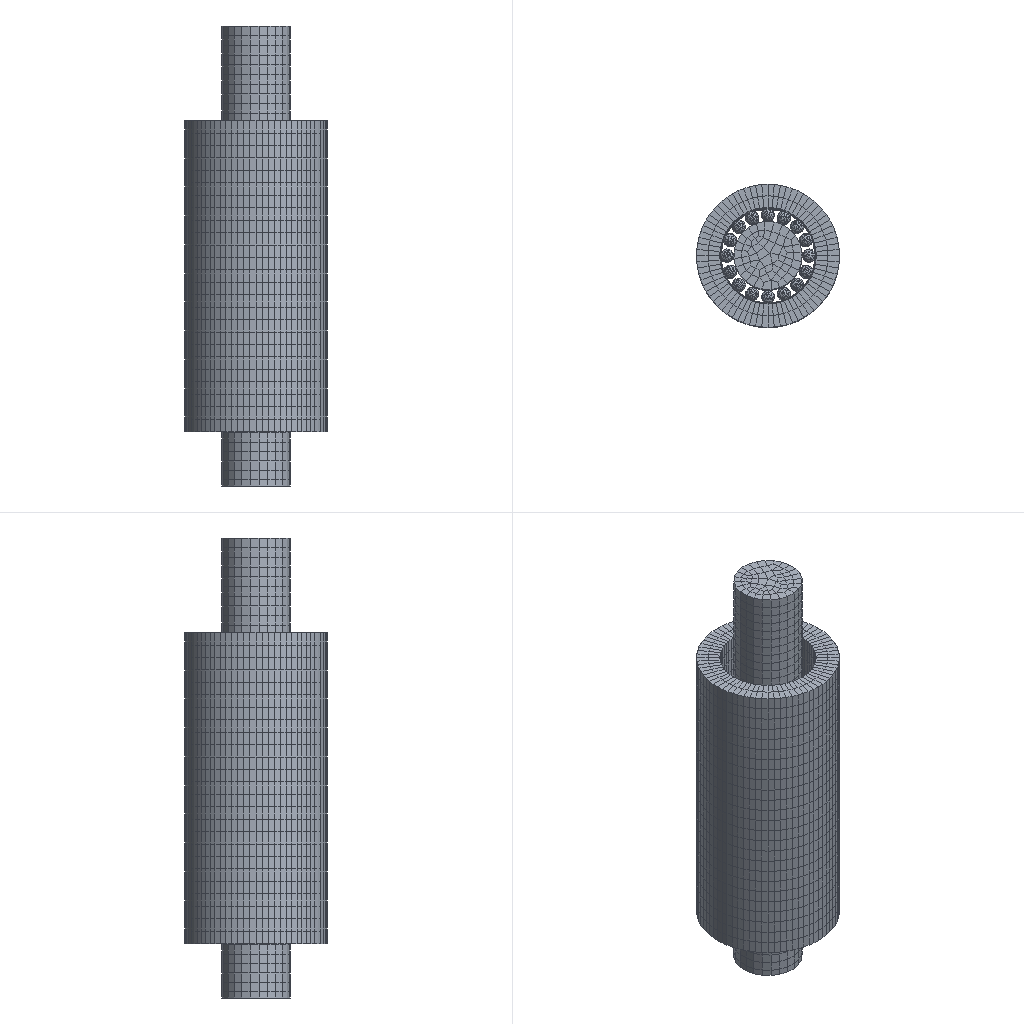Simulation study | abaqus
Set-up summary:
category,name,step,type,value,unit,region
solver,abaqus
solver,version,,,Abaqus/Explicit 2020
units,not stated in the deck,,not stated
analysis,deck,,transient,transient
load_step,Step-1,Step-1,transient
load_step,requested,,,1
mesh,nodes,,,38616
mesh,elements,,,24212
element_type,C3D10,,solid,17427
element_type,C3D8R,,solid,6785
load,load commands in deck,,count,1
bc,support commands in deck,,count,7
material,STEEL,,in results
material,TUBE,,in results
check,setup vs results,,match,"per instance, exact: element labels, types and connectivity; labels of the nodes the elements use; coordinates of those nodes at SINGLE_PRECISION in 2 of 34 instance(s)"
Abaqus input file, long lists of numbers shortened:
*Heading
** Job name: Job-1 Model name: Model-1
** Generated by: Abaqus/CAE 2020
*Preprint, echo=NO, model=NO, history=NO, contact=NO
**
** PARTS
**
*Part, name=work-1
*End Part
**
*Part, name=work-2
*End Part
**
*Part, name=work-3
*End Part
**
*Part, name=work-4
*End Part
**
*Part, name=work-5
*End Part
**
*Part, name=work-6
*End Part
**
*Part, name=work-7
*End Part
**
*Part, name=work-8
*End Part
**
*Part, name=work-9
*End Part
**
*Part, name=work-10
*End Part
**
*Part, name=work-11
*End Part
**
*Part, name=work-12
*End Part
**
*Part, name=work-13
*End Part
**
*Part, name=work-14
*End Part
**
*Part, name=work-15
*End Part
**
*Part, name=work-16
*End Part
**
*Part, name=work-19
*End Part
**
*Part, name=work-20
*End Part
**
*Part, name=work-21
*End Part
**
*Part, name=work-22
*End Part
**
*Part, name=work-23
*End Part
**
*Part, name=work-24
*End Part
**
*Part, name=work-25
*End Part
**
*Part, name=work-26
*End Part
**
*Part, name=work-27
*End Part
**
*Part, name=work-28
*End Part
**
*Part, name=work-29
*End Part
**
*Part, name=work-30
*End Part
**
*Part, name=work-31
*End Part
**
*Part, name=work-32
*End Part
**
*Part, name=work-33
*End Part
**
*Part, name=work-34
*End Part
**
*Part, name=work-35
*End Part
**
*Part, name=work-36
*End Part
**
**
** ASSEMBLY
**
*Assembly, name=Assembly
**
*Instance, name=work-1-1, part=work-1
*Node
      1,   2.556,   14.529,  -2.36
      2,   2.556,   18.529,  -2.36
** (886 more lines like these left out)
*Element, type=C3D10
  1,  84,  38,  85,  42, 142, 141, 140, 144, 143, 145
  2,  84,  86,  87,  88, 148, 147, 146, 150, 149, 151
** (528 more lines like these left out)
*Nset, nset=Set-1, generate
   1,  888,    1
*Elset, elset=Set-1, generate
   1,  530,    1
** Section: steel
*Solid Section, elset=Set-1, material=steel
,
*End Instance
**
*Instance, name=work-2-1, part=work-2
*Node
      1,   6.766,   13.692,  -2.36
      2,   8.296,   17.387,  -2.36
** (769 more lines like these left out)
*Element, type=C3D10
  1,  80,  81,  14,  82, 127, 126, 125, 129, 128, 130
  2,  11,  80,  83,  84, 133, 132, 131, 135, 134, 136
** (445 more lines like these left out)
*Nset, nset=Set-1, generate
   1,  771,    1
*Elset, elset=Set-1, generate
   1,  447,    1
** Section: steel
*Solid Section, elset=Set-1, material=steel
,
*End Instance
**
*Instance, name=work-3-1, part=work-3
*Node
      1,   10.334,   11.307,  -2.36
      2,   13.163,   14.136,  -2.36
** (854 more lines like these left out)
*Element, type=C3D10
  1,  82,  83,  84,  85, 138, 137, 136, 140, 139, 141
  2,  86,  87,  88,  82, 144, 143, 142, 146, 145, 147
** (506 more lines like these left out)
*Nset, nset=Set-1, generate
   1,  856,    1
*Elset, elset=Set-1, generate
   1,  508,    1
** Section: steel
*Solid Section, elset=Set-1, material=steel
,
*End Instance
**
*Instance, name=work-4-1, part=work-4
*Node
      1,   12.719,   7.738,  -2.36
      2,   16.414,   9.269,  -2.36
** (1014 more lines like these left out)
*Element, type=C3D10
  1,   85,   39,    8,   86,  159,  158,  157,  161,  160,  162
  2,   86,   87,   88,   89,  165,  164,  163,  167,  166,  168
** (621 more lines like these left out)
*Nset, nset=Set-1, generate
    1,  1016,     1
*Elset, elset=Set-1, generate
   1,  623,    1
** Section: steel
*Solid Section, elset=Set-1, material=steel
,
*End Instance
**
*Instance, name=work-5-1, part=work-5
*Node
      1,   13.556,   3.529,  -2.36
      2,   17.556,   3.529,  -2.36
** (743 more lines like these left out)
*Element, type=C3D10
  1,  78,  79,  80,  81, 123, 122, 121, 125, 124, 126
  2,  82,  78,  79,  80, 128, 123, 127, 129, 121, 122
** (429 more lines like these left out)
*Nset, nset=Set-1, generate
   1,  745,    1
*Elset, elset=Set-1, generate
   1,  431,    1
** Section: steel
*Solid Section, elset=Set-1, material=steel
,
*End Instance
**
*Instance, name=work-6-1, part=work-6
*Node
      1,   12.719, -0.6806,  -2.36
      2,   16.414,  -2.211,  -2.36
** (875 more lines like these left out)
*Element, type=C3D10
  1,  85,  86,  87,  88, 141, 140, 139, 143, 142, 144
  2,  89,  90,  91,  92, 147, 146, 145, 149, 148, 150
** (518 more lines like these left out)
*Nset, nset=Set-1, generate
   1,  877,    1
*Elset, elset=Set-1, generate
   1,  520,    1
** Section: steel
*Solid Section, elset=Set-1, material=steel
,
*End Instance
**
*Instance, name=work-7-1, part=work-7
*Node
      1,   10.334,  -4.249,  -2.36
      2,   13.163,  -7.078,  -2.36
** (970 more lines like these left out)
*Element, type=C3D10
  1,  88,  89,  90,  91, 154, 153, 152, 156, 155, 157
  2,  88,  92,  93,  94, 160, 159, 158, 162, 161, 163
** (584 more lines like these left out)
*Nset, nset=Set-1, generate
   1,  972,    1
*Elset, elset=Set-1, generate
   1,  586,    1
** Section: steel
*Solid Section, elset=Set-1, material=steel
,
*End Instance
**
*Instance, name=work-8-1, part=work-8
*Node
      1,   6.766,  -6.634,  -2.36
      2,   8.296,  -10.329,  -2.36
** (871 more lines like these left out)
*Element, type=C3D10
  1,   7,  30,  33,  83, 140, 139, 138, 142, 141, 143
  2,  83,  84,  85,  86, 146, 145, 144, 148, 147, 149
** (518 more lines like these left out)
*Nset, nset=Set-1, generate
   1,  873,    1
*Elset, elset=Set-1, generate
   1,  520,    1
** Section: steel
*Solid Section, elset=Set-1, material=steel
,
*End Instance
**
*Instance, name=work-9-1, part=work-9
*Node
      1,   2.556,  -7.471,  -2.36
      2,   2.556,  -11.471,  -2.36
** (858 more lines like these left out)
*Element, type=C3D10
  1,  80,  81,  82,  83, 138, 137, 136, 140, 139, 141
  2,  84,  36,  83,  81, 144, 143, 142, 146, 145, 139
** (512 more lines like these left out)
*Nset, nset=Set-1, generate
   1,  860,    1
*Elset, elset=Set-1, generate
   1,  514,    1
** Section: steel
*Solid Section, elset=Set-1, material=steel
,
*End Instance
**
*Instance, name=work-10-1, part=work-10
*Node
      1,  -1.653,  -6.634,  -2.36
      2,  -3.184,  -10.329,  -2.36
** (794 more lines like these left out)
*Element, type=C3D10
  1,  82,  83,  64,  63, 130, 129, 128, 132, 131, 133
  2,  82,  83,  84,  85, 130, 135, 134, 137, 136, 138
** (462 more lines like these left out)
*Nset, nset=Set-1, generate
   1,  796,    1
*Elset, elset=Set-1, generate
   1,  464,    1
** Section: steel
*Solid Section, elset=Set-1, material=steel
,
*End Instance
**
*Instance, name=work-11-1, part=work-11
*Node
      1,  -5.222,  -4.249,  -2.36
      2,  -8.05,  -7.078,  -2.36
** (759 more lines like these left out)
*Element, type=C3D10
  1,  85,  25,  86,  19, 127, 126, 125, 129, 128, 130
  2,  85,  87,  88,  89, 133, 132, 131, 135, 134, 136
** (430 more lines like these left out)
*Nset, nset=Set-1, generate
   1,  761,    1
*Elset, elset=Set-1, generate
   1,  432,    1
** Section: steel
*Solid Section, elset=Set-1, material=steel
,
*End Instance
**
*Instance, name=work-12-1, part=work-12
*Node
      1,  -7.606, -0.6806,  -2.36
      2,  -11.302,  -2.211,  -2.36
** (760 more lines like these left out)
*Element, type=C3D10
  1,  77,  59,  78,  79, 125, 124, 123, 127, 126, 128
  2,  77,  80,  59,  58, 130, 129, 125, 132, 131, 133
** (443 more lines like these left out)
*Nset, nset=Set-1, generate
   1,  762,    1
*Elset, elset=Set-1, generate
   1,  445,    1
** Section: steel
*Solid Section, elset=Set-1, material=steel
,
*End Instance
**
*Instance, name=work-13-1, part=work-13
*Node
      1,  -8.444,   3.529,  -2.36
      2,  -12.444,   3.529,  -2.36
** (788 more lines like these left out)
*Element, type=C3D10
  1,  83,  84,  52,  85, 130, 129, 128, 132, 131, 133
  2,  83,  77,  85,  51, 135, 134, 132, 137, 136, 138
** (455 more lines like these left out)
*Nset, nset=Set-1, generate
   1,  790,    1
*Elset, elset=Set-1, generate
   1,  457,    1
** Section: steel
*Solid Section, elset=Set-1, material=steel
,
*End Instance
**
*Instance, name=work-14-1, part=work-14
*Node
      1,  -7.606,   7.738,  -2.36
      2,  -11.302,   9.269,  -2.36
** (897 more lines like these left out)
*Element, type=C3D10
  1,  83,  84,  30,  85, 143, 142, 141, 145, 144, 146
  2,  83,  86,  87,  88, 149, 148, 147, 151, 150, 152
** (538 more lines like these left out)
*Nset, nset=Set-1, generate
   1,  899,    1
*Elset, elset=Set-1, generate
   1,  540,    1
** Section: steel
*Solid Section, elset=Set-1, material=steel
,
*End Instance
**
*Instance, name=work-15-1, part=work-15
*Node
      1,  -5.222,   11.307,  -2.36
      2,  -8.05,   14.136,  -2.36
** (694 more lines like these left out)
*Element, type=C3D10
  1,  80,  81,  65,   5, 117, 116, 115, 119, 118, 120
  2,  80,  82,  83,  62, 123, 122, 121, 125, 124, 126
** (390 more lines like these left out)
*Nset, nset=Set-1, generate
   1,  696,    1
*Elset, elset=Set-1, generate
   1,  392,    1
** Section: steel
*Solid Section, elset=Set-1, material=steel
,
*End Instance
**
*Instance, name=work-16-1, part=work-16
*Node
      1,  -1.653,   13.692,  -2.36
      2,  -3.184,   17.387,  -2.36
** (873 more lines like these left out)
*Element, type=C3D10
  1,  84,  32,  85,  36, 141, 140, 139, 143, 142, 144
  2,  84,  86,  85,  42, 146, 145, 139, 148, 147, 149
** (517 more lines like these left out)
*Nset, nset=Set-1, generate
   1,  875,    1
*Elset, elset=Set-1, generate
   1,  519,    1
** Section: steel
*Solid Section, elset=Set-1, material=steel
,
*End Instance
**
*Instance, name=gan, part=work-19
          0.,           0.,         -10.
*Node
      1,   6.328,  -6.804,  -19.891
      2,  -1.215,   13.862,  -19.891
** (3898 more lines like these left out)
*Element, type=C3D8R
   1,  233,   29,   30,  209, 1461,  306,  307, 1437
   2,  230,  231,    1,    9, 1458, 1459,   31,  726
** (3183 more lines like these left out)
*Nset, nset=Set-1, generate
    1,  3900,     1
*Elset, elset=Set-1, generate
    1,  3185,     1
** Section: steel
*Solid Section, elset=Set-1, material=steel
,
*End Instance
**
*Instance, name=tube, part=work-20
          0.,           0.,          30.
*Node
      1,   2.556,   26.529,  -44.36
      2,   25.556,   3.529,  -44.36
** (5614 more lines like these left out)
*Element, type=C3D8R
  1,  114,  681, 4053,  663,    1,   25,  629,   60
  2,  681,  682, 4054, 4053,   25,   26,  630,  629
** (3598 more lines like these left out)
*Nset, nset=Set-1, generate
    1,  5616,     1
*Elset, elset=Set-1, generate
    1,  3600,     1
** Section: tube
*Solid Section, elset=Set-1, material=tube
,
*End Instance
**
*Instance, name=work-21-1, part=work-21
*Node
      1,   2.556,   14.529,   53.39
      2,   2.556,   19.029,   53.39
** (969 more lines like these left out)
*Element, type=C3D10
  1,  86,  87,  88,  89, 153, 152, 151, 155, 154, 156
  2,  90,  86,  91,  92, 159, 158, 157, 161, 160, 162
** (587 more lines like these left out)
*Nset, nset=Set-1, generate
   1,  971,    1
*Elset, elset=Set-1, generate
   1,  589,    1
** Section: steel
*Solid Section, elset=Set-1, material=steel
,
*End Instance
**
*Instance, name=work-22-1, part=work-22
*Node
      1,   6.766,   13.692,   53.39
      2,   8.488,   17.849,   53.39
** (922 more lines like these left out)
*Element, type=C3D10
  1,  86,  87,  88,  89, 148, 147, 146, 150, 149, 151
  2,  86,  88,  76,  90, 146, 153, 152, 155, 154, 156
** (550 more lines like these left out)
*Nset, nset=Set-1, generate
   1,  924,    1
*Elset, elset=Set-1, generate
   1,  552,    1
** Section: steel
*Solid Section, elset=Set-1, material=steel
,
*End Instance
**
*Instance, name=work-23-1, part=work-23
*Node
      1,   10.334,   11.307,   53.39
      2,   13.516,   14.489,   53.39
** (953 more lines like these left out)
*Element, type=C3D10
  1,  85,  86,  84,   4, 151, 150, 149, 153, 152, 154
  2,  85,  87,  88,  89, 157, 156, 155, 159, 158, 160
** (576 more lines like these left out)
*Nset, nset=Set-1, generate
   1,  955,    1
*Elset, elset=Set-1, generate
   1,  578,    1
** Section: steel
*Solid Section, elset=Set-1, material=steel
,
*End Instance
**
*Instance, name=work-24-1, part=work-24
*Node
      1,   12.719,   7.738,   53.39
      2,   16.876,   9.46,   53.39
** (1065 more lines like these left out)
*Element, type=C3D10
  1,   90,   91,   92,   93,  167,  166,  165,  169,  168,  170
  2,   90,   94,   91,   93,  172,  171,  167,  169,  173,  168
** (651 more lines like these left out)
*Nset, nset=Set-1, generate
    1,  1067,     1
*Elset, elset=Set-1, generate
   1,  653,    1
** Section: steel
*Solid Section, elset=Set-1, material=steel
,
*End Instance
**
*Instance, name=work-25-1, part=work-25
*Node
      1,   13.556,   3.529,   53.39
      2,   18.056,   3.529,   53.39
** (999 more lines like these left out)
*Element, type=C3D10
  1,   87,   88,   16,   14,  158,  157,  156,  160,  159,  161
  2,   87,   89,   90,   91,  164,  163,  162,  166,  165,  167
** (606 more lines like these left out)
*Nset, nset=Set-1, generate
    1,  1001,     1
*Elset, elset=Set-1, generate
   1,  608,    1
** Section: steel
*Solid Section, elset=Set-1, material=steel
,
*End Instance
**
*Instance, name=work-26-1, part=work-26
*Node
      1,   12.719, -0.6806,   53.39
      2,   16.876,  -2.403,   53.39
** (967 more lines like these left out)
*Element, type=C3D10
  1,  11,  85,  86,  87, 153, 152, 151, 155, 154, 156
  2,  88,  87,  86,  89, 158, 156, 157, 160, 159, 161
** (586 more lines like these left out)
*Nset, nset=Set-1, generate
   1,  969,    1
*Elset, elset=Set-1, generate
   1,  588,    1
** Section: steel
*Solid Section, elset=Set-1, material=steel
,
*End Instance
**
*Instance, name=work-27-1, part=work-27
*Node
      1,   10.334,  -4.249,   53.39
      2,   13.516,  -7.431,   53.39
** (1018 more lines like these left out)
*Element, type=C3D10
  1,   87,   88,   89,   90,  160,  159,  158,  162,  161,  163
  2,   91,   92,   93,   94,  166,  165,  164,  168,  167,  169
** (621 more lines like these left out)
*Nset, nset=Set-1, generate
    1,  1020,     1
*Elset, elset=Set-1, generate
   1,  623,    1
** Section: steel
*Solid Section, elset=Set-1, material=steel
,
*End Instance
**
*Instance, name=work-28-1, part=work-28
*Node
      1,   6.766,  -6.634,   53.39
      2,   8.488,  -10.791,   53.39
** (1019 more lines like these left out)
*Element, type=C3D10
  1,   85,   86,   87,   30,  159,  158,  157,  161,  160,  162
  2,   88,   89,   90,   91,  165,  164,  163,  167,  166,  168
** (626 more lines like these left out)
*Nset, nset=Set-1, generate
    1,  1021,     1
*Elset, elset=Set-1, generate
   1,  628,    1
** Section: steel
*Solid Section, elset=Set-1, material=steel
,
*End Instance
**
*Instance, name=work-29-1, part=work-29
*Node
      1,   2.556,  -7.471,   53.39
      2,   2.556,  -11.971,   53.39
** (1137 more lines like these left out)
*Element, type=C3D10
  1,   80,   87,   88,   78,  175,  174,  173,  177,  176,  178
  2,   87,   81,   89,   79,  181,  180,  179,  183,  182,  184
** (710 more lines like these left out)
*Nset, nset=Set-1, generate
    1,  1139,     1
*Elset, elset=Set-1, generate
   1,  712,    1
** Section: steel
*Solid Section, elset=Set-1, material=steel
,
*End Instance
**
*Instance, name=work-30-1, part=work-30
*Node
      1,  -1.653,  -6.634,   53.39
      2,  -3.375,  -10.791,   53.39
** (826 more lines like these left out)
*Element, type=C3D10
  1,  38,  83,  84,  85, 135, 134, 133, 137, 136, 138
  2,  86,  85,  41,  87, 141, 140, 139, 143, 142, 144
** (483 more lines like these left out)
*Nset, nset=Set-1, generate
   1,  828,    1
*Elset, elset=Set-1, generate
   1,  485,    1
** Section: steel
*Solid Section, elset=Set-1, material=steel
,
*End Instance
**
*Instance, name=work-31-1, part=work-31
*Node
      1,  -5.222,  -4.249,   53.39
      2,   -8.404,  -7.431,   53.39
** (1046 more lines like these left out)
*Element, type=C3D10
  1,   89,   90,   91,   92,  164,  163,  162,  166,  165,  167
  2,   93,   94,   95,   90,  170,  169,  168,  172,  171,  173
** (639 more lines like these left out)
*Nset, nset=Set-1, generate
    1,  1048,     1
*Elset, elset=Set-1, generate
   1,  641,    1
** Section: steel
*Solid Section, elset=Set-1, material=steel
,
*End Instance
**
*Instance, name=work-32-1, part=work-32
*Node
      1,  -7.606, -0.6806,   53.39
      2,  -11.764,  -2.403,   53.39
** (969 more lines like these left out)
*Element, type=C3D10
  1,  85,  86,  87,  88, 153, 152, 151, 155, 154, 156
  2,  88,  89,  90,  91, 159, 158, 157, 161, 160, 162
** (588 more lines like these left out)
*Nset, nset=Set-1, generate
   1,  971,    1
*Elset, elset=Set-1, generate
   1,  590,    1
** Section: steel
*Solid Section, elset=Set-1, material=steel
,
*End Instance
**
*Instance, name=work-33-1, part=work-33
*Node
      1,  -8.444,   3.529,   53.39
      2,  -12.944,   3.529,   53.39
** (967 more lines like these left out)
*Element, type=C3D10
  1,  87,  88,  89,  90, 154, 153, 152, 156, 155, 157
  2,  87,  91,  92,  93, 160, 159, 158, 162, 161, 163
** (582 more lines like these left out)
*Nset, nset=Set-1, generate
   1,  969,    1
*Elset, elset=Set-1, generate
   1,  584,    1
** Section: steel
*Solid Section, elset=Set-1, material=steel
,
*End Instance
**
*Instance, name=work-34-1, part=work-34
*Node
      1,  -7.606,   7.738,   53.39
      2,  -11.764,   9.46,   53.39
** (985 more lines like these left out)
*Element, type=C3D10
  1,  86,  87,  88,  89, 155, 154, 153, 157, 156, 158
  2,  86,  90,  87,  89, 160, 159, 155, 157, 161, 156
** (599 more lines like these left out)
*Nset, nset=Set-1, generate
   1,  987,    1
*Elset, elset=Set-1, generate
   1,  601,    1
** Section: steel
*Solid Section, elset=Set-1, material=steel
,
*End Instance
**
*Instance, name=work-35-1, part=work-35
*Node
      1,  -5.222,   11.307,   53.39
      2,   -8.404,   14.489,   53.39
** (906 more lines like these left out)
*Element, type=C3D10
  1,  87,  88,  89,  90, 145, 144, 143, 147, 146, 148
  2,  87,  91,  92,  89, 151, 150, 149, 143, 152, 153
** (539 more lines like these left out)
*Nset, nset=Set-1, generate
   1,  908,    1
*Elset, elset=Set-1, generate
   1,  541,    1
** Section: steel
*Solid Section, elset=Set-1, material=steel
,
*End Instance
**
*Instance, name=work-36-1, part=work-36
*Node
      1,  -1.653,   13.692,   53.39
      2,  -3.375,   17.849,   53.39
** (883 more lines like these left out)
*Element, type=C3D10
  1,  29,  85,  86,  87, 142, 141, 140, 144, 143, 145
  2,  85,  87,  29,  28, 143, 144, 142, 147, 146, 148
** (524 more lines like these left out)
*Nset, nset=Set-1, generate
   1,  885,    1
*Elset, elset=Set-1, generate
   1,  526,    1
** Section: steel
*Solid Section, elset=Set-1, material=steel
,
*End Instance
**
*Node
      1,   2.556,   3.529,   116.109
*Node
      2,   2.556,   3.529,   42.109
*Nset, nset=Set-4, instance=gan
    7,    8,  167,  168,  169,  170,  171,  172,  173,  174,  175,  176,  177,  178,  179,  180
  181,  182,  183,  184,  185,  186,  187,  188, 1363, 1364, 1365, 1366, 1367, 1368, 1369, 1370
** (3 more lines like these left out)
*Elset, elset=Set-4, instance=gan, generate
 3121,  3185,     1
*Nset, nset=Set-6, instance=work-1-1, generate
   1,  888,    1
*Nset, nset=Set-6, instance=work-2-1, generate
   1,  771,    1
*Nset, nset=Set-6, instance=work-4-1, generate
    1,  1016,     1
*Nset, nset=Set-6, instance=work-8-1, generate
   1,  873,    1
*Nset, nset=Set-6, instance=work-16-1, generate
   1,  875,    1
*Nset, nset=Set-6, instance=work-32-1, generate
   1,  971,    1
*Nset, nset=Set-6, instance=work-24-1, generate
    1,  1067,     1
*Nset, nset=Set-6, instance=work-12-1, generate
   1,  762,    1
*Nset, nset=Set-6, instance=work-36-1, generate
   1,  885,    1
*Nset, nset=Set-6, instance=work-28-1, generate
    1,  1021,     1
*Nset, nset=Set-6, instance=work-6-1, generate
   1,  877,    1
*Nset, nset=Set-6, instance=work-10-1, generate
   1,  796,    1
*Nset, nset=Set-6, instance=work-34-1, generate
   1,  987,    1
*Nset, nset=Set-6, instance=work-26-1, generate
   1,  969,    1
*Nset, nset=Set-6, instance=work-14-1, generate
   1,  899,    1
*Nset, nset=Set-6, instance=work-22-1, generate
   1,  924,    1
*Nset, nset=Set-6, instance=work-30-1, generate
   1,  828,    1
*Nset, nset=Set-6, instance=work-3-1, generate
   1,  856,    1
*Nset, nset=Set-6, instance=work-5-1, generate
   1,  745,    1
*Nset, nset=Set-6, instance=work-9-1, generate
   1,  860,    1
*Nset, nset=Set-6, instance=work-33-1, generate
   1,  969,    1
*Nset, nset=Set-6, instance=work-25-1, generate
    1,  1001,     1
*Nset, nset=Set-6, instance=work-13-1, generate
   1,  790,    1
*Nset, nset=Set-6, instance=work-21-1, generate
   1,  971,    1
*Nset, nset=Set-6, instance=work-29-1, generate
    1,  1139,     1
*Nset, nset=Set-6, instance=work-7-1, generate
   1,  972,    1
*Nset, nset=Set-6, instance=work-11-1, generate
   1,  761,    1
*Nset, nset=Set-6, instance=work-35-1, generate
   1,  908,    1
*Nset, nset=Set-6, instance=work-27-1, generate
    1,  1020,     1
*Nset, nset=Set-6, instance=work-15-1, generate
   1,  696,    1
*Nset, nset=Set-6, instance=work-23-1, generate
   1,  955,    1
*Nset, nset=Set-6, instance=work-31-1, generate
    1,  1048,     1
*Elset, elset=Set-6, instance=work-1-1, generate
   1,  530,    1
*Elset, elset=Set-6, instance=work-2-1, generate
   1,  447,    1
*Elset, elset=Set-6, instance=work-4-1, generate
   1,  623,    1
*Elset, elset=Set-6, instance=work-8-1, generate
   1,  520,    1
*Elset, elset=Set-6, instance=work-16-1, generate
   1,  519,    1
*Elset, elset=Set-6, instance=work-32-1, generate
   1,  590,    1
*Elset, elset=Set-6, instance=work-24-1, generate
   1,  653,    1
*Elset, elset=Set-6, instance=work-12-1, generate
   1,  445,    1
*Elset, elset=Set-6, instance=work-36-1, generate
   1,  526,    1
*Elset, elset=Set-6, instance=work-28-1, generate
   1,  628,    1
*Elset, elset=Set-6, instance=work-6-1, generate
   1,  520,    1
*Elset, elset=Set-6, instance=work-10-1, generate
   1,  464,    1
*Elset, elset=Set-6, instance=work-34-1, generate
   1,  601,    1
*Elset, elset=Set-6, instance=work-26-1, generate
   1,  588,    1
*Elset, elset=Set-6, instance=work-14-1, generate
   1,  540,    1
*Elset, elset=Set-6, instance=work-22-1, generate
   1,  552,    1
*Elset, elset=Set-6, instance=work-30-1, generate
   1,  485,    1
*Elset, elset=Set-6, instance=work-3-1, generate
   1,  508,    1
*Elset, elset=Set-6, instance=work-5-1, generate
   1,  431,    1
*Elset, elset=Set-6, instance=work-9-1, generate
   1,  514,    1
*Elset, elset=Set-6, instance=work-33-1, generate
   1,  584,    1
*Elset, elset=Set-6, instance=work-25-1, generate
   1,  608,    1
*Elset, elset=Set-6, instance=work-13-1, generate
   1,  457,    1
*Elset, elset=Set-6, instance=work-21-1, generate
   1,  589,    1
*Elset, elset=Set-6, instance=work-29-1, generate
   1,  712,    1
*Elset, elset=Set-6, instance=work-7-1, generate
   1,  586,    1
*Elset, elset=Set-6, instance=work-11-1, generate
   1,  432,    1
*Elset, elset=Set-6, instance=work-35-1, generate
   1,  541,    1
*Elset, elset=Set-6, instance=work-27-1, generate
   1,  623,    1
*Elset, elset=Set-6, instance=work-15-1, generate
   1,  392,    1
*Elset, elset=Set-6, instance=work-23-1, generate
   1,  578,    1
*Elset, elset=Set-6, instance=work-31-1, generate
   1,  641,    1
*Nset, nset=Set-8
 1,
*Nset, nset=Set-11
 2,
*Nset, nset=Set-12, instance=gan, generate
 1363,  1416,     1
*Elset, elset=Set-12, instance=gan, generate
 3121,  3185,     1
*Nset, nset=Set-13, instance=gan
    7,    8,  167,  168,  169,  170,  171,  172,  173,  174,  175,  176,  177,  178,  179,  180
  181,  182,  183,  184,  185,  186,  187,  188, 1363, 1364, 1365, 1366, 1367, 1368, 1369, 1370
** (3 more lines like these left out)
*Elset, elset=Set-13, instance=gan, generate
 3121,  3185,     1
*Nset, nset=m_Set-7
 1,
*Nset, nset=m_Set-10
 2,
*Elset, elset=_s_Surf-1_S2, internal, instance=gan, generate
 3056,  3120,     1
*Surface, type=ELEMENT, name=s_Surf-1
_s_Surf-1_S2, S2
*Elset, elset=_s_Surf-7_S3, internal, instance=work-1-1
   3,  13,  22,  26,  37,  40,  45,  46,  63,  77,  80,  94,  95,  96, 135, 138
 160, 176, 183, 197, 201, 206, 207, 214, 218, 232, 240, 250, 253, 260, 282, 319
** (8 more lines like these left out)
*Elset, elset=_s_Surf-7_S3, internal, instance=work-2-1
  30,  33,  36,  56,  68,  72,  78,  92,  94, 102, 140, 145, 155, 162, 165, 173
 189, 198, 200, 212, 213, 229, 236, 257, 269, 272, 277, 280, 282, 283, 285, 286
** (7 more lines like these left out)
*Elset, elset=_s_Surf-7_S3, internal, instance=work-4-1
  55,  61,  80, 121, 137, 170, 183, 218, 228, 229, 246, 248, 292, 313, 319, 320
 344, 351, 361, 362, 408, 412, 419, 434, 435, 436, 437, 439, 441, 442, 443, 445
** (7 more lines like these left out)
*Elset, elset=_s_Surf-7_S3, internal, instance=work-8-1
   6,  42,  44,  51,  76,  86, 115, 137, 138, 140, 151, 175, 178, 183, 196, 197
 240, 266, 272, 297, 301, 324, 327, 328, 329, 330, 336, 340, 341, 342, 343, 344
** (8 more lines like these left out)
*Elset, elset=_s_Surf-7_S3, internal, instance=work-16-1
  72,  85,  94, 107, 117, 127, 132, 135, 137, 151, 185, 193, 195, 196, 214, 221
 238, 258, 286, 295, 297, 346, 348, 350, 351, 352, 354, 355, 357, 358, 359, 360
** (7 more lines like these left out)
*Elset, elset=_s_Surf-7_S3, internal, instance=work-32-1
  28,  54,  58,  71,  73,  77,  84,  92,  94, 121, 140, 156, 169, 180, 192, 203
 225, 226, 234, 240, 250, 275, 288, 297, 300, 324, 342, 356, 375, 379, 389, 395
** (8 more lines like these left out)
*Elset, elset=_s_Surf-7_S3, internal, instance=work-24-1
  31,  35,  43,  74, 114, 120, 139, 143, 147, 171, 218, 222, 242, 253, 259, 266
 277, 314, 326, 333, 341, 345, 350, 362, 374, 387, 405, 408, 412, 421, 462, 464
** (8 more lines like these left out)
*Elset, elset=_s_Surf-7_S3, internal, instance=work-12-1
  46,  48,  56,  85,  88,  95, 106, 108, 114, 135, 153, 171, 176, 178, 206, 212
 226, 238, 243, 244, 259, 267, 271, 273, 274, 276, 277, 278, 280, 284, 286, 287
** (6 more lines like these left out)
*Elset, elset=_s_Surf-7_S3, internal, instance=work-36-1
  23,  37,  70,  77,  80,  92, 108, 137, 145, 150, 151, 218, 229, 233, 238, 244
 253, 267, 279, 285, 286, 294, 301, 314, 326, 338, 340, 343, 344, 345, 346, 347
** (7 more lines like these left out)
*Elset, elset=_s_Surf-7_S3, internal, instance=work-28-1
  13,  29,  42,  57,  69,  72, 108, 110, 112, 137, 140, 156, 164, 204, 206, 214
 218, 226, 243, 266, 275, 293, 299, 331, 343, 348, 394, 400, 412, 416, 425, 461
** (8 more lines like these left out)
*Elset, elset=_s_Surf-7_S3, internal, instance=work-6-1
  25,  39,  63,  88, 108, 115, 125, 129, 131, 138, 172, 180, 199, 214, 234, 254
 266, 274, 279, 283, 288, 310, 312, 315, 326, 340, 343, 344, 349, 350, 351, 353
** (7 more lines like these left out)
*Elset, elset=_s_Surf-7_S3, internal, instance=work-10-1
  46,  57,  74,  80,  86, 107, 116, 126, 137, 145, 199, 205, 207, 217, 226, 244
 246, 253, 258, 262, 263, 264, 267, 272, 275, 276, 277, 283, 287, 288, 289, 290
** (7 more lines like these left out)
*Elset, elset=_s_Surf-7_S3, internal, instance=work-34-1
  29,  60,  61,  68,  78,  92, 106, 112, 114, 139, 140, 155, 183, 215, 253, 263
 267, 281, 283, 285, 290, 300, 326, 332, 378, 403, 408, 410, 411, 412, 413, 414
** (8 more lines like these left out)
*Elset, elset=_s_Surf-7_S3, internal, instance=work-26-1
  13,  26,  37,  39,  44,  51,  57,  58,  60,  66,  98, 101, 124, 126, 140, 164
 172, 218, 221, 237, 247, 261, 310, 315, 329, 341, 368, 370, 371, 387, 392, 399
** (8 more lines like these left out)
*Elset, elset=_s_Surf-7_S3, internal, instance=work-14-1
  12,  30,  37,  51,  54,  73,  81,  95, 116, 126, 134, 140, 161, 200, 207, 259
 278, 300, 303, 321, 345, 355, 358, 360, 362, 363, 364, 365, 366, 367, 368, 369
** (7 more lines like these left out)
*Elset, elset=_s_Surf-7_S3, internal, instance=work-22-1
  29,  37,  50,  68,  83, 102, 110, 124, 137, 160, 177, 184, 197, 206, 214, 217
 220, 241, 259, 283, 288, 334, 366, 374, 379, 387, 388, 389, 390, 392, 394, 396
** (7 more lines like these left out)
*Elset, elset=_s_Surf-7_S3, internal, instance=work-30-1
   3,   7,   8,  31,  35,  44,  45,  58,  63,  73, 112, 131, 183, 202, 225, 240
 259, 269, 277, 300, 306, 319, 321, 322, 324, 325, 327, 328, 329, 330, 331, 333
** (7 more lines like these left out)
*Elset, elset=_s_Surf-7_S3, internal, instance=work-3-1
  25,  48,  95,  98,  99, 113, 121, 126, 134, 139, 160, 187, 193, 200, 218, 228
 236, 238, 257, 285, 292, 311, 319, 333, 334, 335, 336, 337, 338, 339, 340, 341
** (8 more lines like these left out)
*Elset, elset=_s_Surf-7_S3, internal, instance=work-5-1
  43,  51,  54,  55,  58,  60,  76,  85,  89, 111, 113, 115, 118, 119, 132, 148
 177, 180, 201, 213, 218, 220, 241, 244, 252, 260, 261, 267, 268, 269, 271, 282
** (7 more lines like these left out)
*Elset, elset=_s_Surf-7_S3, internal, instance=work-9-1
  37, 110, 112, 125, 136, 138, 142, 156, 206, 207, 218, 236, 258, 277, 279, 309
 310, 340, 344, 347, 348, 350, 351, 353, 354, 355, 356, 357, 358, 360, 361, 362
** (7 more lines like these left out)
*Elset, elset=_s_Surf-7_S3, internal, instance=work-33-1
  32,  36,  37,  56,  58,  80,  92, 109, 152, 178, 182, 192, 209, 212, 276, 292
 300, 305, 321, 329, 331, 356, 363, 364, 387, 394, 401, 407, 412, 413, 414, 416
** (8 more lines like these left out)
*Elset, elset=_s_Surf-7_S3, internal, instance=work-25-1
  11,  18,  22,  23,  27,  55,  98, 107, 111, 114, 118, 140, 143, 153, 154, 205
 218, 228, 231, 253, 276, 299, 305, 325, 327, 341, 357, 362, 373, 377, 403, 412
** (8 more lines like these left out)
*Elset, elset=_s_Surf-7_S3, internal, instance=work-13-1
  47,  54,  61,  65,  71,  75,  98, 108, 109, 110, 114, 117, 137, 138, 141, 148
 154, 164, 202, 207, 213, 244, 254, 261, 270, 271, 274, 275, 276, 277, 280, 282
** (7 more lines like these left out)
*Elset, elset=_s_Surf-7_S3, internal, instance=work-21-1
  37,  63,  66,  71,  83,  97, 131, 137, 150, 165, 183, 204, 215, 217, 226, 228
 239, 262, 264, 272, 287, 289, 290, 309, 324, 337, 345, 364, 367, 371, 378, 379
** (7 more lines like these left out)
*Elset, elset=_s_Surf-7_S3, internal, instance=work-29-1
   3,  49,  54,  55,  58,  61,  77,  85,  89, 112, 118, 174, 195, 214, 236, 239
 242, 252, 300, 334, 345, 373, 377, 383, 385, 392, 398, 400, 401, 408, 412, 413
** (7 more lines like these left out)
*Elset, elset=_s_Surf-7_S3, internal, instance=work-7-1
  25,  37,  72, 151, 211, 213, 217, 239, 240, 251, 252, 260, 271, 316, 317, 332
 342, 351, 360, 367, 372, 373, 375, 376, 377, 379, 380, 382, 383, 384, 385, 386
** (8 more lines like these left out)
*Elset, elset=_s_Surf-7_S3, internal, instance=work-11-1
  19,  21,  47,  61,  80,  84, 136, 137, 138, 140, 148, 149, 234, 235, 237, 238
 239, 242, 244, 245, 246, 247, 250, 251, 252, 253, 254, 255, 256, 257, 258, 259
** (8 more lines like these left out)
*Elset, elset=_s_Surf-7_S3, internal, instance=work-35-1
  10,  40,  49,  68,  94, 100, 101, 106, 116, 134, 145, 161, 188, 193, 213, 214
 227, 248, 263, 267, 275, 279, 280, 310, 326, 332, 340, 341, 345, 346, 363, 364
** (8 more lines like these left out)
*Elset, elset=_s_Surf-7_S3, internal, instance=work-27-1
  17,  33,  45,  70, 101, 108, 114, 115, 116, 125, 138, 175, 214, 216, 218, 229
 236, 274, 305, 309, 326, 357, 359, 361, 364, 383, 406, 419, 425, 426, 434, 447
** (8 more lines like these left out)
*Elset, elset=_s_Surf-7_S3, internal, instance=work-15-1
  24,  29,  77,  90,  92, 113, 116, 121, 123, 135, 167, 190, 191, 192, 193, 194
 195, 196, 197, 198, 201, 202, 204, 205, 206, 207, 208, 209, 210, 211, 212, 213
** (7 more lines like these left out)
*Elset, elset=_s_Surf-7_S3, internal, instance=work-23-1
 148, 175, 178, 187, 199, 207, 214, 215, 218, 222, 249, 277, 281, 299, 303, 337
 362, 363, 386, 402, 403, 404, 405, 406, 407, 408, 409, 410, 413, 415, 417, 418
** (8 more lines like these left out)
*Elset, elset=_s_Surf-7_S3, internal, instance=work-31-1
  36,  37,  52,  77,  93,  95, 100, 101, 111, 169, 175, 183, 199, 206, 207, 213
 216, 220, 227, 261, 267, 276, 286, 293, 305, 323, 343, 351, 357, 374, 386, 399
** (8 more lines like these left out)
*Elset, elset=_s_Surf-7_S1, internal, instance=work-1-1
 226,
*Elset, elset=_s_Surf-7_S1, internal, instance=work-4-1
  45, 293, 306, 566
*Elset, elset=_s_Surf-7_S1, internal, instance=work-8-1
   1, 281
*Elset, elset=_s_Surf-7_S1, internal, instance=work-16-1
 145, 194, 271, 333, 408
*Elset, elset=_s_Surf-7_S1, internal, instance=work-32-1
 282, 319, 352, 367, 404
*Elset, elset=_s_Surf-7_S1, internal, instance=work-24-1
 430,
*Elset, elset=_s_Surf-7_S1, internal, instance=work-12-1
 110, 214, 246, 253, 269, 400, 410, 434
*Elset, elset=_s_Surf-7_S1, internal, instance=work-36-1
  28,  68,  79, 115, 240, 364, 444
*Elset, elset=_s_Surf-7_S1, internal, instance=work-28-1
 314, 338, 340, 345, 527
*Elset, elset=_s_Surf-7_S1, internal, instance=work-6-1
  27, 179, 313, 394
*Elset, elset=_s_Surf-7_S1, internal, instance=work-10-1
 68, 78
*Elset, elset=_s_Surf-7_S1, internal, instance=work-34-1
 185, 249, 393, 559
*Elset, elset=_s_Surf-7_S1, internal, instance=work-26-1
 109, 246, 258, 332, 335, 558
*Elset, elset=_s_Surf-7_S1, internal, instance=work-14-1
  66,  68,  72, 291, 312, 455, 462, 482, 513
*Elset, elset=_s_Surf-7_S1, internal, instance=work-22-1
  22,  31, 318, 324, 344
*Elset, elset=_s_Surf-7_S1, internal, instance=work-30-1
 258, 318
*Elset, elset=_s_Surf-7_S1, internal, instance=work-3-1
  34, 168
*Elset, elset=_s_Surf-7_S1, internal, instance=work-5-1
  63, 188, 193, 231, 251, 277, 283
*Elset, elset=_s_Surf-7_S1, internal, instance=work-9-1
  54,  71, 146, 149, 328, 511
*Elset, elset=_s_Surf-7_S1, internal, instance=work-33-1
  39, 325, 371, 405
*Elset, elset=_s_Surf-7_S1, internal, instance=work-25-1
 223, 352, 394, 530
*Elset, elset=_s_Surf-7_S1, internal, instance=work-13-1
 102, 189
*Elset, elset=_s_Surf-7_S1, internal, instance=work-21-1
  96, 168, 197, 336
*Elset, elset=_s_Surf-7_S1, internal, instance=work-29-1
 433, 485, 546, 698
*Elset, elset=_s_Surf-7_S1, internal, instance=work-7-1
 124, 178, 374, 458
*Elset, elset=_s_Surf-7_S1, internal, instance=work-11-1
 147, 159, 173, 222, 236
*Elset, elset=_s_Surf-7_S1, internal, instance=work-35-1
  25, 114, 208, 247, 386, 466
*Elset, elset=_s_Surf-7_S1, internal, instance=work-27-1
 150, 308, 349, 387
*Elset, elset=_s_Surf-7_S1, internal, instance=work-15-1
  30,  74, 111, 126
*Elset, elset=_s_Surf-7_S1, internal, instance=work-23-1
  18, 198, 292
*Elset, elset=_s_Surf-7_S1, internal, instance=work-31-1
 353, 370, 589
*Elset, elset=_s_Surf-7_S4, internal, instance=work-1-1
 113, 242, 255, 281, 320, 455, 466, 479
*Elset, elset=_s_Surf-7_S4, internal, instance=work-2-1
  27,  61, 219, 235, 249, 274, 314, 321, 338, 342, 391
*Elset, elset=_s_Surf-7_S4, internal, instance=work-4-1
  94, 162, 212, 304, 348, 410, 422, 465, 511, 553, 573, 599, 621
*Elset, elset=_s_Surf-7_S4, internal, instance=work-8-1
 164, 294, 355, 410
*Elset, elset=_s_Surf-7_S4, internal, instance=work-16-1
   9,  18,  90, 113, 206, 245, 250, 307, 322, 406, 439, 456, 469, 497, 514
*Elset, elset=_s_Surf-7_S4, internal, instance=work-32-1
 110, 308, 332, 418, 440, 543, 559, 568
*Elset, elset=_s_Surf-7_S4, internal, instance=work-24-1
 116, 224, 318, 332, 439, 481, 494, 502, 555, 608
*Elset, elset=_s_Surf-7_S4, internal, instance=work-12-1
  60, 145, 158, 191, 297, 428, 440
*Elset, elset=_s_Surf-7_S4, internal, instance=work-36-1
   6,  32,  83, 259, 272, 316, 339, 342, 379, 403, 458, 459, 509
*Elset, elset=_s_Surf-7_S4, internal, instance=work-28-1
 116, 197, 222, 292, 377, 396, 575, 623
*Elset, elset=_s_Surf-7_S4, internal, instance=work-6-1
  34,  60, 136, 331, 382, 465, 501
*Elset, elset=_s_Surf-7_S4, internal, instance=work-10-1
   8,  13, 160, 174, 209, 273, 279, 342
*Elset, elset=_s_Surf-7_S4, internal, instance=work-34-1
  91,  94, 203, 293, 380, 431, 459
*Elset, elset=_s_Surf-7_S4, internal, instance=work-26-1
  95, 103, 144, 161, 269, 331, 430, 480, 585
*Elset, elset=_s_Surf-7_S4, internal, instance=work-14-1
 132, 137, 251, 253, 260, 282, 383, 427, 516, 517
*Elset, elset=_s_Surf-7_S4, internal, instance=work-22-1
 115, 135, 159, 164, 167, 189, 195, 238, 261, 275, 285, 457, 499, 523
*Elset, elset=_s_Surf-7_S4, internal, instance=work-30-1
   6,  89, 158, 169, 205, 226, 254, 303, 378, 384, 401, 416, 422, 455, 459
*Elset, elset=_s_Surf-7_S4, internal, instance=work-3-1
  76, 264, 328
*Elset, elset=_s_Surf-7_S4, internal, instance=work-5-1
  32,  83,  86, 144, 198, 226, 237, 287
*Elset, elset=_s_Surf-7_S4, internal, instance=work-9-1
  34, 186, 190, 301, 311, 317, 370, 402, 403, 439, 462
*Elset, elset=_s_Surf-7_S4, internal, instance=work-33-1
  20, 183, 410, 426, 449, 452
*Elset, elset=_s_Surf-7_S4, internal, instance=work-25-1
 328, 345, 348, 379, 423, 438, 497, 602
*Elset, elset=_s_Surf-7_S4, internal, instance=work-13-1
 143, 146, 196, 211, 291, 415
*Elset, elset=_s_Surf-7_S4, internal, instance=work-21-1
 138, 280, 299, 312, 352, 381, 391, 415, 430, 473, 499, 534
*Elset, elset=_s_Surf-7_S4, internal, instance=work-29-1
  35,  41,  43, 102, 161, 169, 278, 341, 394, 437, 448, 490, 524, 531, 581, 627
*Elset, elset=_s_Surf-7_S4, internal, instance=work-7-1
  43, 305, 318, 322, 324, 369
*Elset, elset=_s_Surf-7_S4, internal, instance=work-11-1
  28, 123, 206, 216, 291, 295, 325, 348, 391, 410
*Elset, elset=_s_Surf-7_S4, internal, instance=work-35-1
  13,  43, 156, 330, 351, 378, 397, 427, 448, 487, 489, 533
*Elset, elset=_s_Surf-7_S4, internal, instance=work-27-1
  88, 130, 301, 332, 458, 474, 520, 532, 581, 588
*Elset, elset=_s_Surf-7_S4, internal, instance=work-15-1
  85, 105, 128, 302, 333, 391
*Elset, elset=_s_Surf-7_S4, internal, instance=work-23-1
 226, 242, 273, 321, 462, 481, 488, 510, 576
*Elset, elset=_s_Surf-7_S4, internal, instance=work-31-1
 136, 163, 426, 572, 628, 633
*Elset, elset=_s_Surf-7_S2, internal, instance=work-1-1
 382, 388
*Elset, elset=_s_Surf-7_S2, internal, instance=work-2-1
 290, 316, 336, 349, 352, 354, 382, 395, 407, 418
*Elset, elset=_s_Surf-7_S2, internal, instance=work-4-1
 175, 192, 364, 536, 549
*Elset, elset=_s_Surf-7_S2, internal, instance=work-8-1
 382, 387, 396, 443, 514
*Elset, elset=_s_Surf-7_S2, internal, instance=work-16-1
  41, 234, 349, 389, 415, 482, 483, 512
*Elset, elset=_s_Surf-7_S2, internal, instance=work-32-1
 224, 359, 489, 518, 539, 548
*Elset, elset=_s_Surf-7_S2, internal, instance=work-24-1
 403, 495, 506, 520, 597, 615, 631
*Elset, elset=_s_Surf-7_S2, internal, instance=work-12-1
 266, 275, 291, 374, 376, 384, 421
*Elset, elset=_s_Surf-7_S2, internal, instance=work-36-1
 415, 428, 470, 477, 481, 487
*Elset, elset=_s_Surf-7_S2, internal, instance=work-28-1
  85, 557, 581, 611, 616
*Elset, elset=_s_Surf-7_S2, internal, instance=work-6-1
 352, 354, 362, 383, 403, 426, 453, 464, 489, 511
*Elset, elset=_s_Surf-7_S2, internal, instance=work-10-1
 271, 369, 404, 460
*Elset, elset=_s_Surf-7_S2, internal, instance=work-34-1
 192, 433, 449, 489, 549, 555, 593
*Elset, elset=_s_Surf-7_S2, internal, instance=work-26-1
 107, 488, 565, 570
*Elset, elset=_s_Surf-7_S2, internal, instance=work-14-1
  25, 162, 166, 524
*Elset, elset=_s_Surf-7_S2, internal, instance=work-22-1
 107, 376, 395, 402, 423, 446, 456, 471, 482, 483, 491, 501, 516
*Elset, elset=_s_Surf-7_S2, internal, instance=work-30-1
  57,  64,  78, 326, 342, 386, 440
*Elset, elset=_s_Surf-7_S2, internal, instance=work-3-1
 351, 352, 368, 415, 442, 479, 504
*Elset, elset=_s_Surf-7_S2, internal, instance=work-5-1
 140, 146, 299, 393, 414, 426
*Elset, elset=_s_Surf-7_S2, internal, instance=work-9-1
 318, 342, 385, 387, 404, 444, 474
*Elset, elset=_s_Surf-7_S2, internal, instance=work-33-1
  60, 469, 474, 513, 535, 561
*Elset, elset=_s_Surf-7_S2, internal, instance=work-25-1
 100, 405, 461, 485, 512, 515, 519, 554
*Elset, elset=_s_Surf-7_S2, internal, instance=work-13-1
 273, 313, 336, 337, 433, 438, 439, 444, 448, 457
*Elset, elset=_s_Surf-7_S2, internal, instance=work-21-1
 459, 477, 524, 525, 554, 565, 586
*Elset, elset=_s_Surf-7_S2, internal, instance=work-29-1
  39, 183, 244, 302, 574, 587, 608, 610, 682
*Elset, elset=_s_Surf-7_S2, internal, instance=work-7-1
 514, 566
*Elset, elset=_s_Surf-7_S2, internal, instance=work-11-1
 307, 315, 361
*Elset, elset=_s_Surf-7_S2, internal, instance=work-35-1
 372, 395, 402, 500, 531
*Elset, elset=_s_Surf-7_S2, internal, instance=work-27-1
  55, 464, 472, 543, 570, 587, 599
*Elset, elset=_s_Surf-7_S2, internal, instance=work-15-1
  79,  89, 328, 375
*Elset, elset=_s_Surf-7_S2, internal, instance=work-23-1
 423, 547, 556, 570
*Elset, elset=_s_Surf-7_S2, internal, instance=work-31-1
  42, 366, 506, 544, 574, 582, 593, 602, 638
*Surface, type=ELEMENT, name=s_Surf-7
_s_Surf-7_S3, S3
_s_Surf-7_S1, S1
_s_Surf-7_S4, S4
_s_Surf-7_S2, S2
*Elset, elset=_s_Surf-9_S5, internal, instance=tube
  19,  20,  21,  22,  23,  24,  25,  26,  27,  28,  29,  30,  31,  32,  33,  34
  35,  36,  55,  56,  57,  58,  59,  60,  61,  62,  63,  64,  65,  66,  67,  68
** (10 more lines like these left out)
*Elset, elset=_s_Surf-9_S4, internal, instance=tube
  362,  364,  366,  368,  370,  372,  374,  376,  378,  380,  382,  384,  386,  388,  390,  392
  394,  396,  398,  400,  402,  404,  406,  408,  410,  412,  414,  416,  418,  420,  422,  424
** (27 more lines like these left out)
*Elset, elset=_s_Surf-9_S2, internal, instance=tube, generate
 2701,  2970,     1
*Elset, elset=_s_Surf-9_S1, internal, instance=tube, generate
 3421,  3600,     1
*Elset, elset=_s_Surf-9_S6, internal, instance=tube
  721,  723,  725,  727,  729,  731,  733,  735,  737,  739,  741,  743,  745,  747,  749,  751
  753,  755,  757,  759,  761,  763,  765,  767,  769,  771,  773,  775,  777,  779,  781,  783
** (43 more lines like these left out)
*Surface, type=ELEMENT, name=s_Surf-9
_s_Surf-9_S5, S5
_s_Surf-9_S4, S4
_s_Surf-9_S2, S2
_s_Surf-9_S6, S6
_s_Surf-9_S1, S1
*Elset, elset=_s_Surf-14_S4, internal, instance=gan
    1,   12,   19,   23,   24,   25,   26,   27,   28,   29,   30,   31,   32,   34,   35,   37
   40,   66,   77,   84,   88,   89,   90,   91,   92,   93,   94,   95,   96,   97,   99,  100
** (41 more lines like these left out)
*Elset, elset=_s_Surf-14_S6, internal, instance=gan
   13,   17,   22,   78,   82,   87,  143,  147,  152,  208,  212,  217,  273,  277,  282,  338
  342,  347,  403,  407,  412,  468,  472,  477,  533,  537,  542,  598,  602,  607,  663,  667
** (6 more lines like these left out)
*Elset, elset=_s_Surf-14_S5, internal, instance=gan
    2,   18,   67,   83,  132,  148,  197,  213,  262,  278,  327,  343,  392,  408,  457,  473
  522,  538,  587,  603,  652,  668,  717,  733,  782,  798,  847,  863,  912,  928,  977,  993
** (3 more lines like these left out)
*Elset, elset=_s_Surf-14_S3, internal, instance=gan
   11,   21,   76,   86,  141,  151,  206,  216,  271,  281,  336,  346,  401,  411,  466,  476
  531,  541,  596,  606,  661,  671,  726,  736,  791,  801,  856,  866,  921,  931,  986,  996
** (3 more lines like these left out)
*Surface, type=ELEMENT, name=s_Surf-14
_s_Surf-14_S4, S4
_s_Surf-14_S6, S6
_s_Surf-14_S5, S5
_s_Surf-14_S3, S3
*Elset, elset=_s_Surf-15_S4, internal, instance=gan
 2601, 2612, 2619, 2623, 2624, 2625, 2626, 2627, 2628, 2629, 2630, 2631, 2632, 2634, 2635, 2637
 2640, 2666, 2677, 2684, 2688, 2689, 2690, 2691, 2692, 2693, 2694, 2695, 2696, 2697, 2699, 2700
** (7 more lines like these left out)
*Elset, elset=_s_Surf-15_S6, internal, instance=gan
 2613, 2617, 2622, 2678, 2682, 2687, 2743, 2747, 2752, 2808, 2812, 2817, 2873, 2877, 2882, 2938
 2942, 2947, 3003, 3007, 3012, 3068, 3072, 3077
*Elset, elset=_s_Surf-15_S5, internal, instance=gan
 2602, 2618, 2667, 2683, 2732, 2748, 2797, 2813, 2862, 2878, 2927, 2943, 2992, 3008, 3057, 3073
*Elset, elset=_s_Surf-15_S2, internal, instance=gan, generate
 3056,  3120,     1
*Elset, elset=_s_Surf-15_S3, internal, instance=gan
 2611, 2621, 2676, 2686, 2741, 2751, 2806, 2816, 2871, 2881, 2936, 2946, 3001, 3011, 3066, 3076
*Surface, type=ELEMENT, name=s_Surf-15
_s_Surf-15_S4, S4
_s_Surf-15_S6, S6
_s_Surf-15_S2, S2
_s_Surf-15_S5, S5
_s_Surf-15_S3, S3
** Constraint: Constraint-1
*Coupling, constraint name=Constraint-1, ref node=m_Set-7, surface=s_Surf-15
*Kinematic
*End Assembly
*Amplitude, name=Amp-1
             0.,              0.,            0.05,              1.
**
** MATERIALS
**
*Material, name=steel
*Density
 7.85e-09,
*Elastic
206000., 0.3
*Material, name=tube
*Density
 7.85e-09,
*Elastic
206000., 0.3
*Plastic
550.,0.
**
** INTERACTION PROPERTIES
**
*Surface Interaction, name=IntProp-1
*Friction
 0.2,
*Surface Behavior, pressure-overclosure=HARD
**
** INTERACTIONS
**
** Interaction: Int-4
*Contact, op=NEW
*Contact Inclusions, ALL EXTERIOR
*Contact Property Assignment
 ,  , IntProp-1
** ----------------------------------------------------------------
**
** STEP: Step-1
**
*Step, name=Step-1, nlgeom=YES
*Dynamic, Explicit
, 0.05
*Bulk Viscosity
0.06, 1.2
** Mass Scaling: Semi-Automatic
**               Whole Model
*Fixed Mass Scaling, factor=500.
**
** BOUNDARY CONDITIONS
**
** Name: BC-1 Type: 对称/反对称/完全固定
*Boundary
Set-13, ENCASTRE
** Name: [REDACTED] : Displacement/rotation angle
*Boundary, amplitude=Amp-1
Set-8, 1, 1
Set-8, 2, 2
Set-8, 3, 3, -20.
Set-8, 4, 4
Set-8, 5, 5
Set-8, 6, 6
**
** OUTPUT REQUESTS
**
*Restart, write, number interval=1, time marks=NO
**
** FIELD OUTPUT: F-Output-1
**
*Output, field
*Node Output
CF, RF, RM, RT, U, V
*Element Output, directions=YES
E, ELEDEN, ELEN, ENER, LE, MISES, MISESMAX, NFORC, PE, PEEQ, S, SF
*Contact Output
CDISP, CSTRESS
**
** HISTORY OUTPUT: H-Output-1
**
*Output, history, time interval=2.5e-05
*Node Output, nset=Set-8
RF3, U3
**
** HISTORY OUTPUT: H-Output-2
**
*Output, history, variable=PRESELECT, time interval=2.5e-05
*End Step
Results summary:
result,step,Step-1,completed,increments=71091 time=0.05/0.05
result,analysis,,,transient
result,last_loadstep,,,1
result,primary field,,,U
result,reaction total,,FX,-806757.942,model units
result,reaction total,,FY,844686.413,model units
result,reaction total,,FZ,112473.644,model units